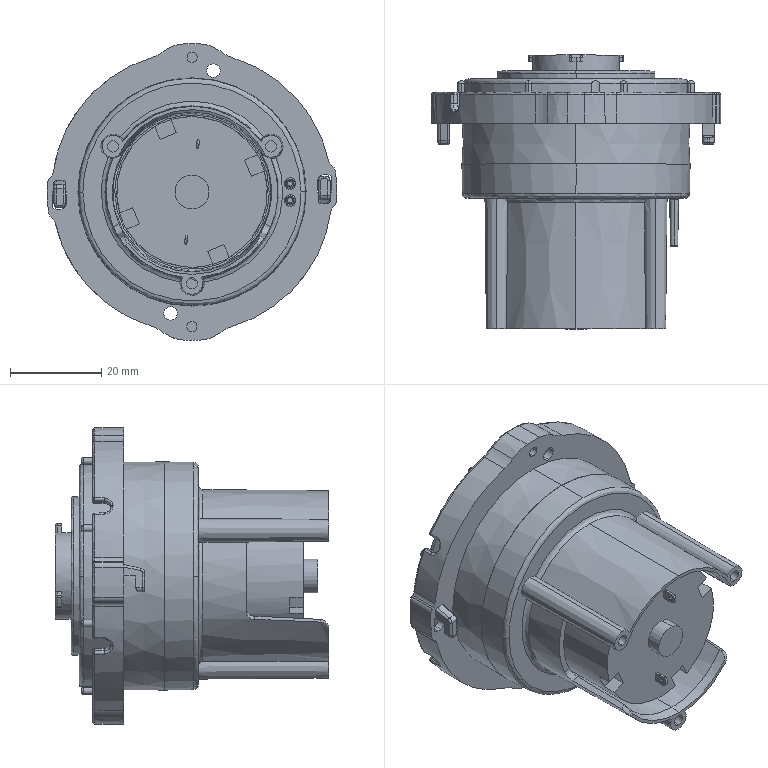Part | SolidWorks | features InContextFeatHolder 3 | 9 solids | 1094 faces | box 63.5 x 60 x 65 mm | volume 47283 mm3 | plane 350 | cylinder 322 | cone 270 | spline 151 | torus 1 | commonest cylinder face diameters 4 x45 1 x32 2.5 x28 1.5 x20 2 x20 5.95 x11